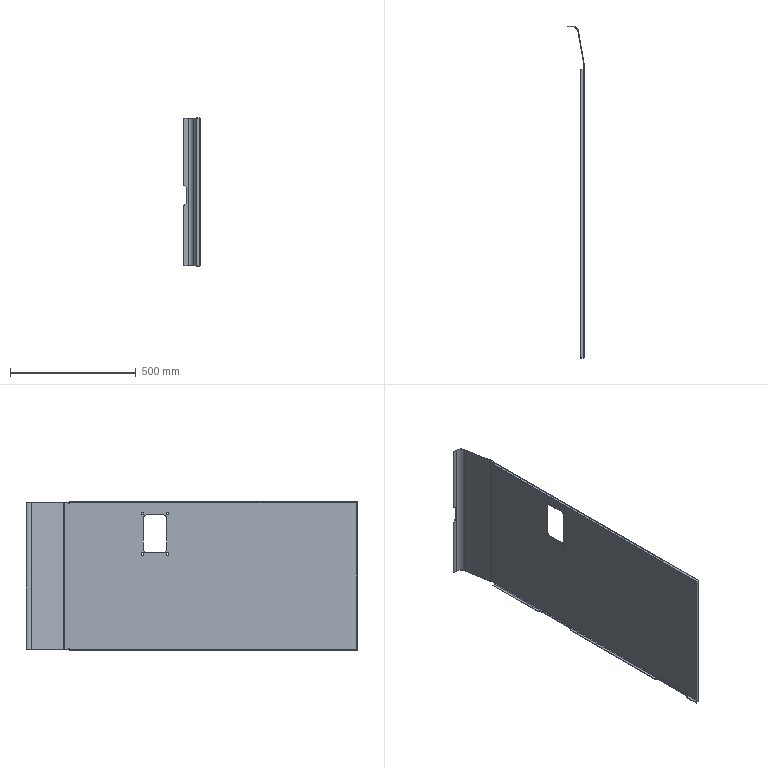Part | SolidWorks | features ICE 4, Chamfer 1, EdgeFlange 1, Fillet 1, FlatPattern 1, SMBaseFlange 1, SheetMetal 1 | 1 solid | 88 faces | box 65.7 x 1318 x 591 mm | volume 1870359 mm3 | plane 52 | cylinder 32 | spline 4 | commonest cylinder face diameters 10 x8 30 x8 20 x4 5 x3 9.6 x3 4 x2